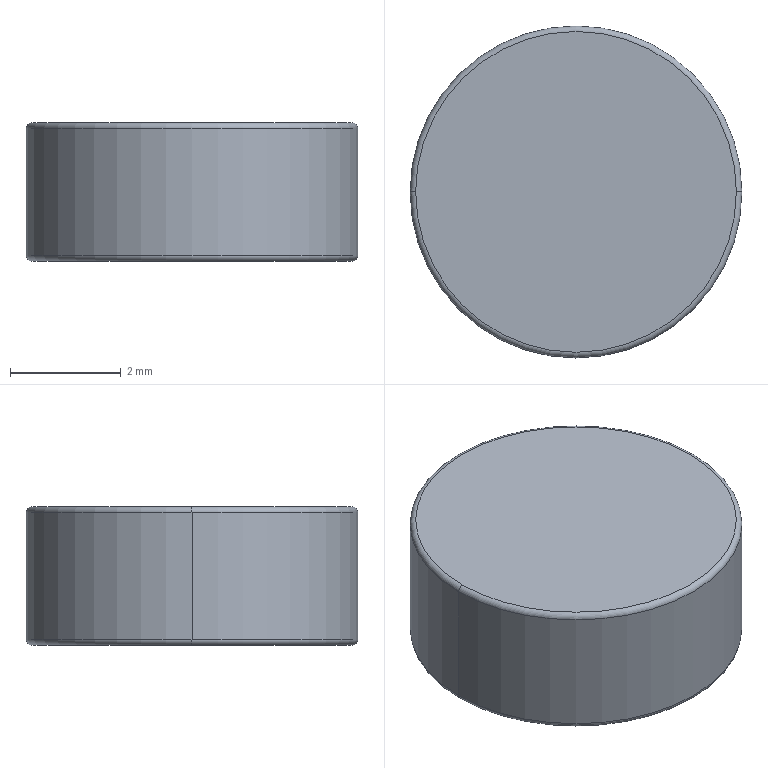Part | NX | features BREP 1 | 1 solid | 8 faces | box 6 x 6 x 2.5 mm | volume 70.606 mm3 | torus 4 | cylinder 2 | plane 2 | commonest cylinder face diameters 6 x2
STEP:
#1=CARTESIAN_POINT('',(-3.,0.,2.4));
#2=VERTEX_POINT('',#1);
#3=CARTESIAN_POINT('',(3.,0.,2.4));
#4=VERTEX_POINT('',#3);
#5=CARTESIAN_POINT('',(0.,0.,2.4));
#6=DIRECTION('',(0.,0.,-1.));
#7=DIRECTION('',(1.,0.,0.));
#8=AXIS2_PLACEMENT_3D('',#5,#6,#7);
#9=CIRCLE('',#8,3.);
#10=EDGE_CURVE('',#2,#4,#9,.T.);
#11=ORIENTED_EDGE('',*,*,#10,.F.);
#12=CARTESIAN_POINT('',(-2.9,0.,2.5));
#13=VERTEX_POINT('',#12);
#14=CARTESIAN_POINT('',(-2.9,0.,2.4));
#15=DIRECTION('',(0.,1.,0.));
#16=DIRECTION('',(-1.,0.,0.));
#17=AXIS2_PLACEMENT_3D('',#14,#15,#16);
#18=CIRCLE('',#17,0.1);
#19=EDGE_CURVE('',#2,#13,#18,.T.);
#20=ORIENTED_EDGE('',*,*,#19,.T.);
#21=CARTESIAN_POINT('',(2.9,0.,2.5));
#22=VERTEX_POINT('',#21);
#23=CARTESIAN_POINT('',(0.,0.,2.5));
#24=DIRECTION('',(0.,0.,1.));
#25=DIRECTION('',(1.,0.,0.));
#26=AXIS2_PLACEMENT_3D('',#23,#24,#25);
#27=CIRCLE('',#26,2.9);
#28=EDGE_CURVE('',#22,#13,#27,.T.);
#29=ORIENTED_EDGE('',*,*,#28,.F.);
#30=CARTESIAN_POINT('',(2.9,0.,2.4));
#31=DIRECTION('',(0.,-1.,0.));
#32=DIRECTION('',(0.,0.,-1.));
#33=AXIS2_PLACEMENT_3D('',#30,#31,#32);
#34=CIRCLE('',#33,0.1);
#35=EDGE_CURVE('',#4,#22,#34,.T.);
#36=ORIENTED_EDGE('',*,*,#35,.F.);
#37=EDGE_LOOP('',(#11,#20,#29,#36));
#38=FACE_BOUND('',#37,.T.);
#39=CARTESIAN_POINT('',(0.,0.,2.4));
#40=DIRECTION('',(0.,0.,1.));
#41=DIRECTION('',(-1.,0.,0.));
#42=AXIS2_PLACEMENT_3D('',#39,#40,#41);
#43=TOROIDAL_SURFACE('',#42,2.9,0.1);
#44=ADVANCED_FACE('',(#38),#43,.T.);
#45=CARTESIAN_POINT('',(-2.9,0.,0.));
#46=VERTEX_POINT('',#45);
#47=CARTESIAN_POINT('',(2.9,0.,0.));
#48=VERTEX_POINT('',#47);
#49=CARTESIAN_POINT('',(0.,0.,0.));
#50=DIRECTION('',(0.,0.,-1.));
#51=DIRECTION('',(1.,0.,0.));
#52=AXIS2_PLACEMENT_3D('',#49,#50,#51);
#53=CIRCLE('',#52,2.9);
#54=EDGE_CURVE('',#46,#48,#53,.T.);
#55=ORIENTED_EDGE('',*,*,#54,.F.);
#56=CARTESIAN_POINT('',(-3.,0.,0.1));
#57=VERTEX_POINT('',#56);
#58=CARTESIAN_POINT('',(-2.9,0.,0.1));
#59=DIRECTION('',(0.,1.,0.));
#60=DIRECTION('',(-1.,0.,0.));
#61=AXIS2_PLACEMENT_3D('',#58,#59,#60);
#62=CIRCLE('',#61,0.1);
#63=EDGE_CURVE('',#46,#57,#62,.T.);
#64=ORIENTED_EDGE('',*,*,#63,.T.);
#65=CARTESIAN_POINT('',(3.,0.,0.1));
#66=VERTEX_POINT('',#65);
#67=CARTESIAN_POINT('',(0.,0.,0.1));
#68=DIRECTION('',(0.,0.,1.));
#69=DIRECTION('',(1.,0.,0.));
#70=AXIS2_PLACEMENT_3D('',#67,#68,#69);
#71=CIRCLE('',#70,3.);
#72=EDGE_CURVE('',#66,#57,#71,.T.);
#73=ORIENTED_EDGE('',*,*,#72,.F.);
#74=CARTESIAN_POINT('',(2.9,0.,0.1));
#75=DIRECTION('',(0.,-1.,0.));
#76=DIRECTION('',(0.,0.,-1.));
#77=AXIS2_PLACEMENT_3D('',#74,#75,#76);
#78=CIRCLE('',#77,0.1);
#79=EDGE_CURVE('',#48,#66,#78,.T.);
#80=ORIENTED_EDGE('',*,*,#79,.F.);
#81=EDGE_LOOP('',(#55,#64,#73,#80));
#82=FACE_BOUND('',#81,.T.);
#83=CARTESIAN_POINT('',(0.,0.,0.1));
#84=DIRECTION('',(0.,0.,1.));
#85=DIRECTION('',(-1.,0.,0.));
#86=AXIS2_PLACEMENT_3D('',#83,#84,#85);
#87=TOROIDAL_SURFACE('',#86,2.9,0.1);
#88=ADVANCED_FACE('',(#82),#87,.T.);
#89=ORIENTED_EDGE('',*,*,#10,.T.);
#90=CARTESIAN_POINT('',(3.,0.,2.5));
#91=DIRECTION('',(0.,0.,-1.));
#92=VECTOR('',#91,1000.);
#93=LINE('',#90,#92);
#94=EDGE_CURVE('',#66,#4,#93,.F.);
#95=ORIENTED_EDGE('',*,*,#94,.F.);
#96=ORIENTED_EDGE('',*,*,#72,.T.);
#97=CARTESIAN_POINT('',(-3.,0.,2.5));
#98=DIRECTION('',(0.,0.,-1.));
#99=VECTOR('',#98,1000.);
#100=LINE('',#97,#99);
#101=EDGE_CURVE('',#57,#2,#100,.F.);
#102=ORIENTED_EDGE('',*,*,#101,.T.);
#103=EDGE_LOOP('',(#89,#95,#96,#102));
#104=FACE_BOUND('',#103,.T.);
#105=CARTESIAN_POINT('',(0.,0.,2.5));
#106=DIRECTION('',(0.,0.,-1.));
#107=DIRECTION('',(1.,0.,0.));
#108=AXIS2_PLACEMENT_3D('',#105,#106,#107);
#109=CYLINDRICAL_SURFACE('',#108,3.);
#110=ADVANCED_FACE('',(#104),#109,.T.);
#111=ORIENTED_EDGE('',*,*,#94,.T.);
#112=CARTESIAN_POINT('',(0.,0.,2.4));
#113=DIRECTION('',(0.,0.,-1.));
#114=DIRECTION('',(1.,0.,0.));
#115=AXIS2_PLACEMENT_3D('',#112,#113,#114);
#116=CIRCLE('',#115,3.);
#117=EDGE_CURVE('',#4,#2,#116,.T.);
#118=ORIENTED_EDGE('',*,*,#117,.T.);
#119=ORIENTED_EDGE('',*,*,#101,.F.);
#120=CARTESIAN_POINT('',(0.,0.,0.1));
#121=DIRECTION('',(0.,0.,1.));
#122=DIRECTION('',(1.,0.,0.));
#123=AXIS2_PLACEMENT_3D('',#120,#121,#122);
#124=CIRCLE('',#123,3.);
#125=EDGE_CURVE('',#57,#66,#124,.T.);
#126=ORIENTED_EDGE('',*,*,#125,.T.);
#127=EDGE_LOOP('',(#111,#118,#119,#126));
#128=FACE_BOUND('',#127,.T.);
#129=CARTESIAN_POINT('',(0.,0.,2.5));
#130=DIRECTION('',(0.,0.,-1.));
#131=DIRECTION('',(1.,0.,0.));
#132=AXIS2_PLACEMENT_3D('',#129,#130,#131);
#133=CYLINDRICAL_SURFACE('',#132,3.);
#134=ADVANCED_FACE('',(#128),#133,.T.);
#135=ORIENTED_EDGE('',*,*,#28,.T.);
#136=CARTESIAN_POINT('',(0.,0.,2.5));
#137=DIRECTION('',(0.,0.,1.));
#138=DIRECTION('',(1.,0.,0.));
#139=AXIS2_PLACEMENT_3D('',#136,#137,#138);
#140=CIRCLE('',#139,2.9);
#141=EDGE_CURVE('',#13,#22,#140,.T.);
#142=ORIENTED_EDGE('',*,*,#141,.T.);
#143=EDGE_LOOP('',(#135,#142));
#144=FACE_BOUND('',#143,.T.);
#145=CARTESIAN_POINT('',(0.,0.,2.5));
#146=DIRECTION('',(0.,0.,1.));
#147=DIRECTION('',(-1.,0.,0.));
#148=AXIS2_PLACEMENT_3D('',#145,#146,#147);
#149=PLANE('',#148);
#150=ADVANCED_FACE('',(#144),#149,.T.);
#151=CARTESIAN_POINT('',(0.,0.,0.));
#152=DIRECTION('',(0.,0.,-1.));
#153=DIRECTION('',(1.,0.,0.));
#154=AXIS2_PLACEMENT_3D('',#151,#152,#153);
#155=CIRCLE('',#154,2.9);
#156=EDGE_CURVE('',#48,#46,#155,.T.);
#157=ORIENTED_EDGE('',*,*,#156,.T.);
#158=ORIENTED_EDGE('',*,*,#54,.T.);
#159=EDGE_LOOP('',(#157,#158));
#160=FACE_BOUND('',#159,.T.);
#161=CARTESIAN_POINT('',(0.,0.,0.));
#162=DIRECTION('',(0.,0.,1.));
#163=DIRECTION('',(-1.,0.,0.));
#164=AXIS2_PLACEMENT_3D('',#161,#162,#163);
#165=PLANE('',#164);
#166=ADVANCED_FACE('',(#160),#165,.F.);
#167=ORIENTED_EDGE('',*,*,#63,.F.);
#168=ORIENTED_EDGE('',*,*,#156,.F.);
#169=ORIENTED_EDGE('',*,*,#79,.T.);
#170=ORIENTED_EDGE('',*,*,#125,.F.);
#171=EDGE_LOOP('',(#167,#168,#169,#170));
#172=FACE_BOUND('',#171,.T.);
#173=CARTESIAN_POINT('',(0.,0.,0.1));
#174=DIRECTION('',(0.,0.,1.));
#175=DIRECTION('',(-1.,0.,0.));
#176=AXIS2_PLACEMENT_3D('',#173,#174,#175);
#177=TOROIDAL_SURFACE('',#176,2.9,0.1);
#178=ADVANCED_FACE('',(#172),#177,.T.);
#179=ORIENTED_EDGE('',*,*,#19,.F.);
#180=ORIENTED_EDGE('',*,*,#117,.F.);
#181=ORIENTED_EDGE('',*,*,#35,.T.);
#182=ORIENTED_EDGE('',*,*,#141,.F.);
#183=EDGE_LOOP('',(#179,#180,#181,#182));
#184=FACE_BOUND('',#183,.T.);
#185=CARTESIAN_POINT('',(0.,0.,2.4));
#186=DIRECTION('',(0.,0.,1.));
#187=DIRECTION('',(-1.,0.,0.));
#188=AXIS2_PLACEMENT_3D('',#185,#186,#187);
#189=TOROIDAL_SURFACE('',#188,2.9,0.1);
#190=ADVANCED_FACE('',(#184),#189,.T.);
#191=CLOSED_SHELL('',(#44,#88,#110,#134,#150,#166,#178,#190));
#192=MANIFOLD_SOLID_BREP('',#191);
#193=(LENGTH_UNIT()NAMED_UNIT(*)SI_UNIT(.MILLI.,.METRE.));
#194=UNCERTAINTY_MEASURE_WITH_UNIT(LENGTH_MEASURE(0.00001),#193,'','');
#195=(NAMED_UNIT(*)PLANE_ANGLE_UNIT()SI_UNIT($,.RADIAN.));
#196=(NAMED_UNIT(*)SI_UNIT($,.STERADIAN.)SOLID_ANGLE_UNIT());
#197=(GEOMETRIC_REPRESENTATION_CONTEXT(3)GLOBAL_UNCERTAINTY_ASSIGNED_CONTEXT((#194))GLOBAL_UNIT_ASSIGNED_CONTEXT((#193,#195,#196))REPRESENTATION_CONTEXT('',''));
#198=ADVANCED_BREP_SHAPE_REPRESENTATION('',(#192),#197);